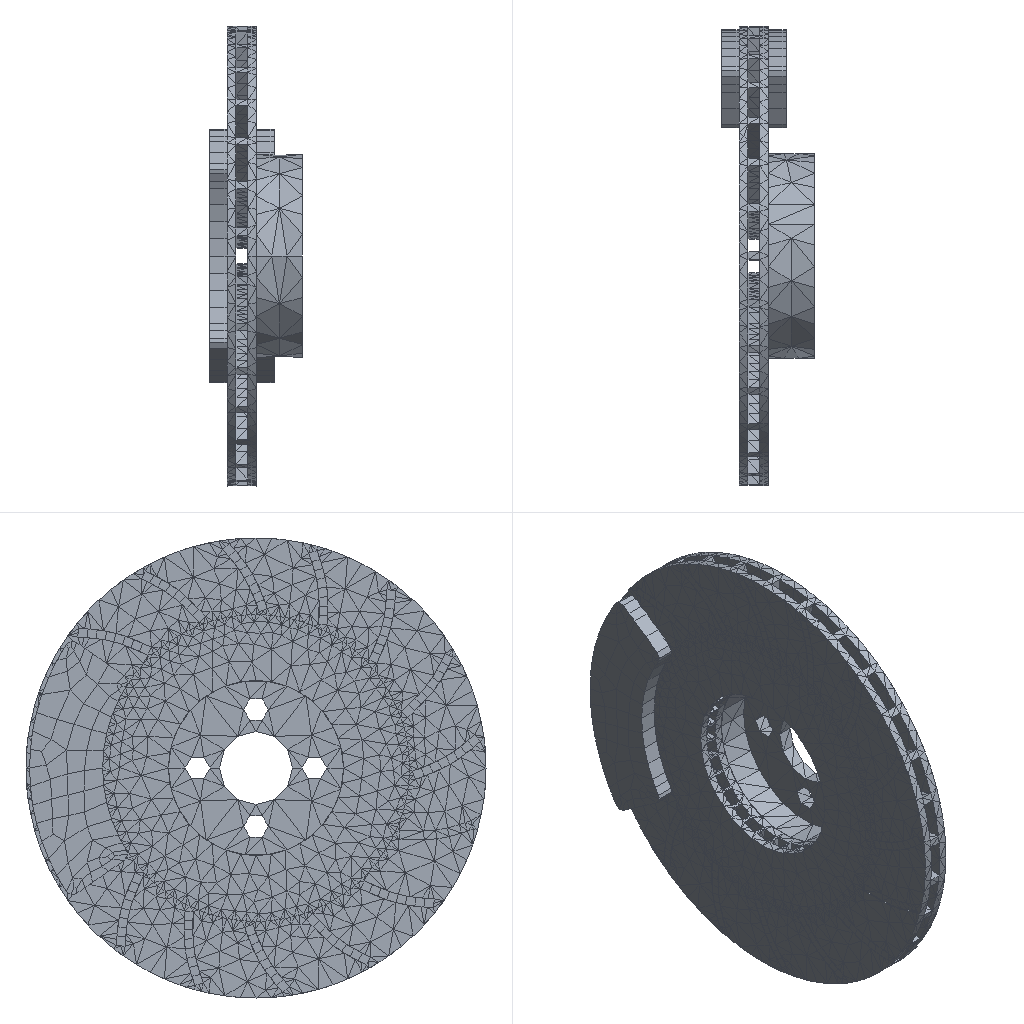Simulation study | ansys workbench
Set-up summary:
category,name,step,type,value,unit,region
solver,ansys_workbench
units,mm-N-s-tonne (MPa),,stated,"/units,MPA"
analysis,deck-1/LS1,,transient thermal
load_step,deck-1/LS1,deck-1/LS1,transient thermal,nsubst=100; time=1
analysis,deck-2/LS1,,static
load_step,deck-2/LS1,deck-2/LS1,static,nsubst=1; time=1
mesh,deck-1.dat,,nodes,28738
mesh,deck-1.dat,,elements,19638
element_type,SOLID291,,,13218,,deck-1.dat
element_type,TARGE170,,,2148,,deck-1.dat
element_type,CONTA174,,,2148,,deck-1.dat
element_type,SURF152,,,1858,,deck-1.dat
element_type,SOLID279,,,266,,deck-1.dat
mesh,deck-2.dat,,nodes,28738
mesh,deck-2.dat,,elements,17780
element_type,SOLID187,,,13218,,deck-2.dat
element_type,TARGE170,,,2148,,deck-2.dat
element_type,CONTA174,,,2148,,deck-2.dat
element_type,SOLID186,,,266,,deck-2.dat
material,Structural Steel,,E,200000,tonne s^-2 mm^-1
material,Structural Steel,,nu,0.3
material,Structural Steel,,density,7.85e-09,tonne mm^-3
material,Structural Steel,,conductivity,60.5,tonne mm s^-3 C^-1
material,Structural Steel,,specific_heat,4.34e+08,mm^2 s^-2 C^-1
material,Structural Steel,,cte,1.2e-05,C^-1
material,Structural Steel,,permeability,10000
material,Structural Steel,,resistivity,0.00017,ohm mm
load,Define Uniform Initial temperature,deck-1/model,body load temp,22,,all
load,"Create ""______""",deck-1/LS1,convection,15000,,SURF152 #62
bc,,deck-1/LS1,temperature,200 [dofs=TEMP],,node list
bc,Fixed Supports,deck-2/model,fixed,[dofs=ALL],,_FIXEDSU
contact,Contact Region,,bonded (always),element=CONTA174
contact,Contact Region 2,,bonded (always),element=CONTA174
contact,Contact Region 3,,bonded (always),element=CONTA174
contact,Contact Region 4,,bonded (always),element=CONTA174
contact,Contact Region 5,,bonded (always),element=CONTA174
contact,Contact Region 6,,bonded (always),element=CONTA174
contact,Contact Region 7,,bonded (always),element=CONTA174
contact,Contact Region 8,,bonded (always),element=CONTA174
contact,Contact Region 9,,bonded (always),element=CONTA174
contact,Contact Region 10,,bonded (always),element=CONTA174
contact,Contact Region 11,,bonded (always),element=CONTA174
contact,Contact Region 12,,bonded (always),element=CONTA174
contact,Contact Region 13,,bonded (always),element=CONTA174
contact,Contact Region 14,,bonded (always),element=CONTA174
contact,Contact Region 15,,bonded (always),element=CONTA174
contact,Contact Region 16,,bonded (always),element=CONTA174
contact,Contact Region 17,,bonded (always),element=CONTA174
contact,Contact Region 18,,bonded (always),element=CONTA174
contact,Contact Region 19,,bonded (always),element=CONTA174
contact,Contact Region 20,,bonded (always),element=CONTA174
contact,Contact Region 21,,bonded (always),element=CONTA174
contact,Contact Region,,bonded (always),element=CONTA174
contact,Contact Region 2,,bonded (always),element=CONTA174
contact,Contact Region 3,,bonded (always),element=CONTA174
contact,Contact Region 4,,bonded (always),element=CONTA174
contact,Contact Region 5,,bonded (always),element=CONTA174
contact,Contact Region 6,,bonded (always),element=CONTA174
contact,Contact Region 7,,bonded (always),element=CONTA174
contact,Contact Region 8,,bonded (always),element=CONTA174
contact,Contact Region 9,,bonded (always),element=CONTA174
contact,Contact Region 10,,bonded (always),element=CONTA174
contact,Contact Region 11,,bonded (always),element=CONTA174
contact,Contact Region 12,,bonded (always),element=CONTA174
contact,Contact Region 13,,bonded (always),element=CONTA174
contact,Contact Region 14,,bonded (always),element=CONTA174
contact,Contact Region 15,,bonded (always),element=CONTA174
contact,Contact Region 16,,bonded (always),element=CONTA174
contact,Contact Region 17,,bonded (always),element=CONTA174
contact,Contact Region 18,,bonded (always),element=CONTA174
contact,Contact Region 19,,bonded (always),element=CONTA174
contact,Contact Region 20,,bonded (always),element=CONTA174
contact,Contact Region 21,,bonded (always),element=CONTA174
named_set,_CM151,,node,4828
named_set,_FIXEDSU,,node,216
gap,"BFBLOCK present, not parsed (28738 lines)"
Results summary:
result,analyses[0].index,,,1
result,analyses[0].system,,,SYS
result,analyses[0].deck,,,deck-1.dat
result,analyses[0].solve_status,,,completed
result,analyses[0].analysis_type,,,static
result,analyses[0].physics,,,thermal
result,analyses[0].unit_system,,,"NMM: mm, ton, N, s, mV, mA, degC"
result,analyses[0].n_sets,,,17
result,analyses[0].load_steps[0].set,set=17,,17
result,analyses[0].load_steps[0].time_or_freq,set=17,,1
result,analyses[0].load_steps[0].max_temperature,set=17,,221.25
result,analyses[0].load_steps[0].min_temperature,set=17,,11.576
result,analyses[1].index,,,2
result,analyses[1].system,,,SYS-1
result,analyses[1].deck,,,deck-2.dat
result,analyses[1].solve_status,,,completed
result,analyses[1].analysis_type,,,static
result,analyses[1].physics,,,mechanical
result,analyses[1].unit_system,,,"NMM: mm, ton, N, s, mV, mA, degC"
result,analyses[1].n_sets,,,1
result,analyses[1].load_steps[0].set,set=1,,1
result,analyses[1].load_steps[0].time_or_freq,set=1,,1
result,analyses[1].load_steps[0].max_displacement_magnitude,set=1,,0.2323
result,analyses[1].load_steps[0].max_von_mises_nodal,set=1,,699.155
result,analyses[1].load_steps[0].reaction_force_sum_xyz[1],set=1,,-1.04223e-07
result,analyses[1].load_steps[0].reaction_force_sum_xyz[2],set=1,,7.36549e-09
result,analyses[1].load_steps[0].reaction_force_sum_xyz[3],set=1,,-7.23509e-08